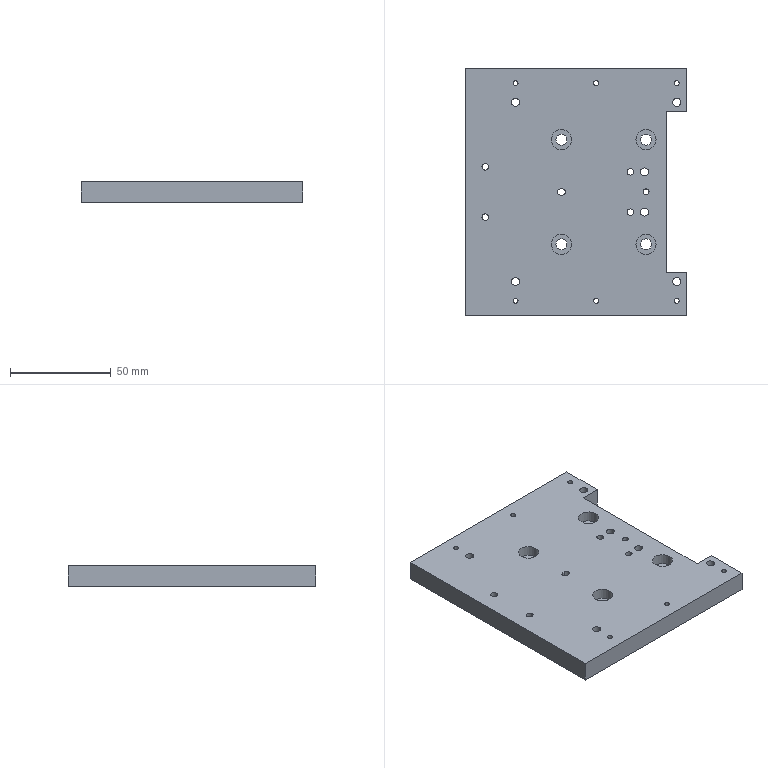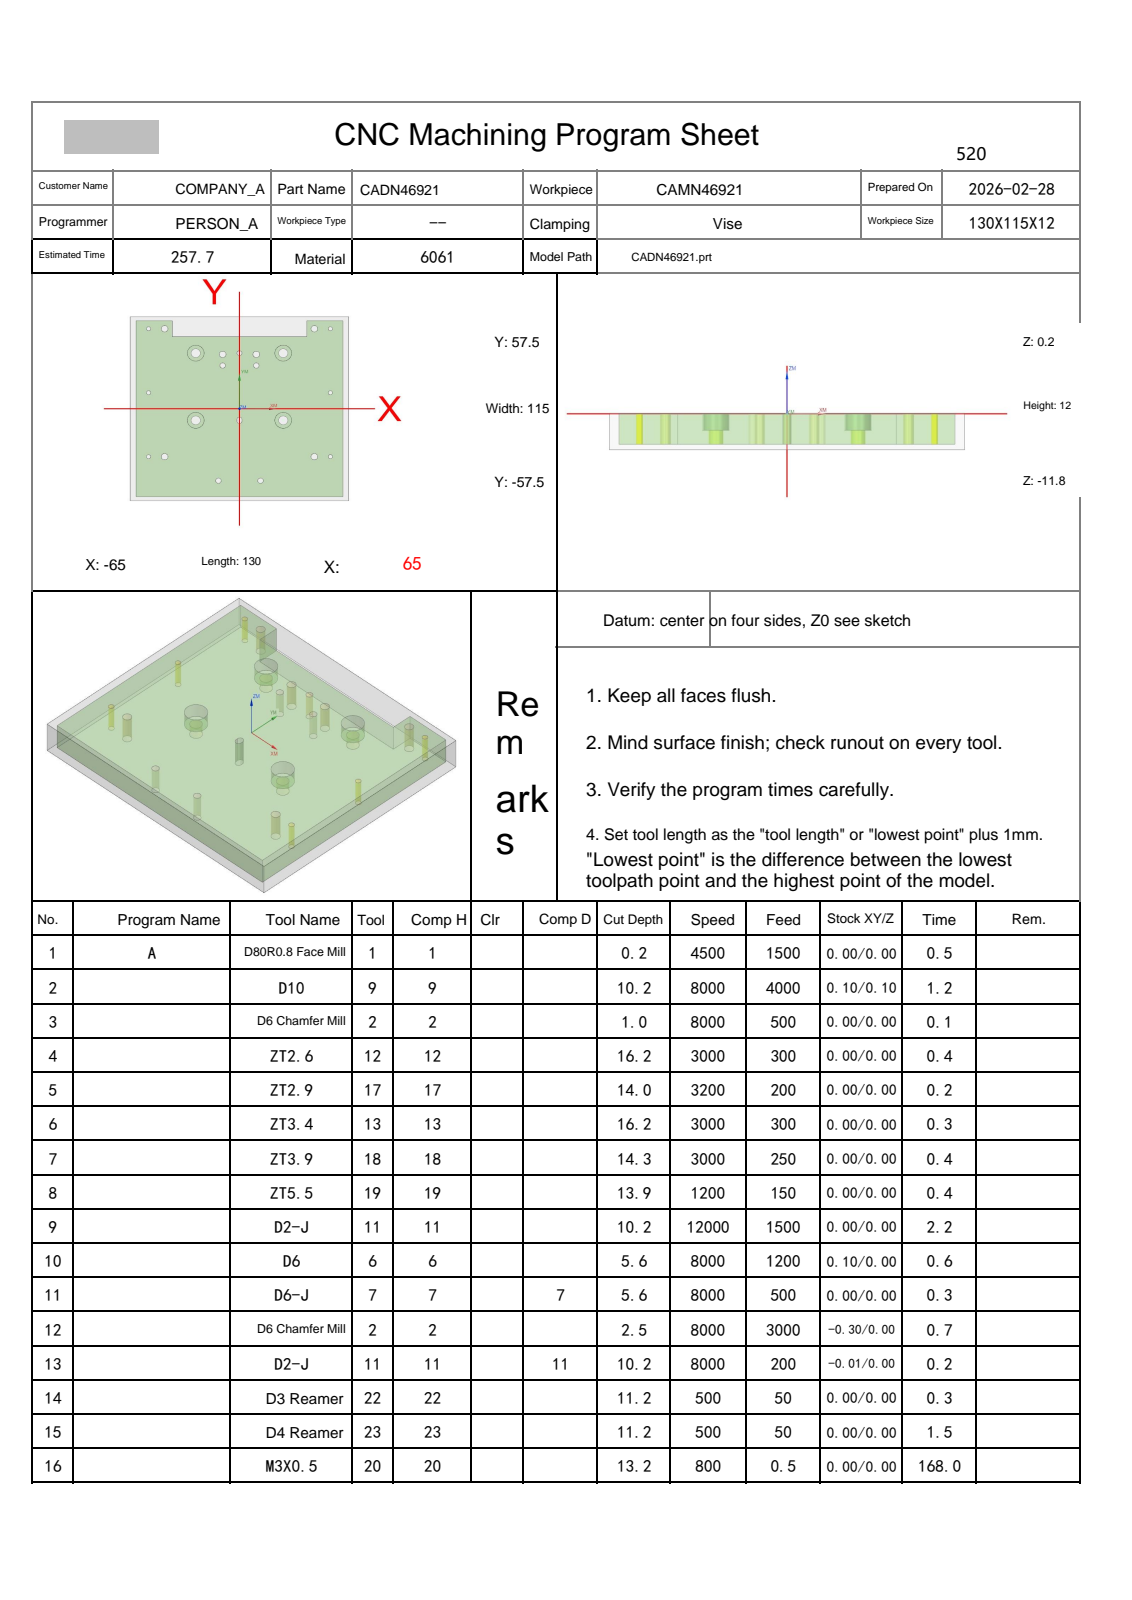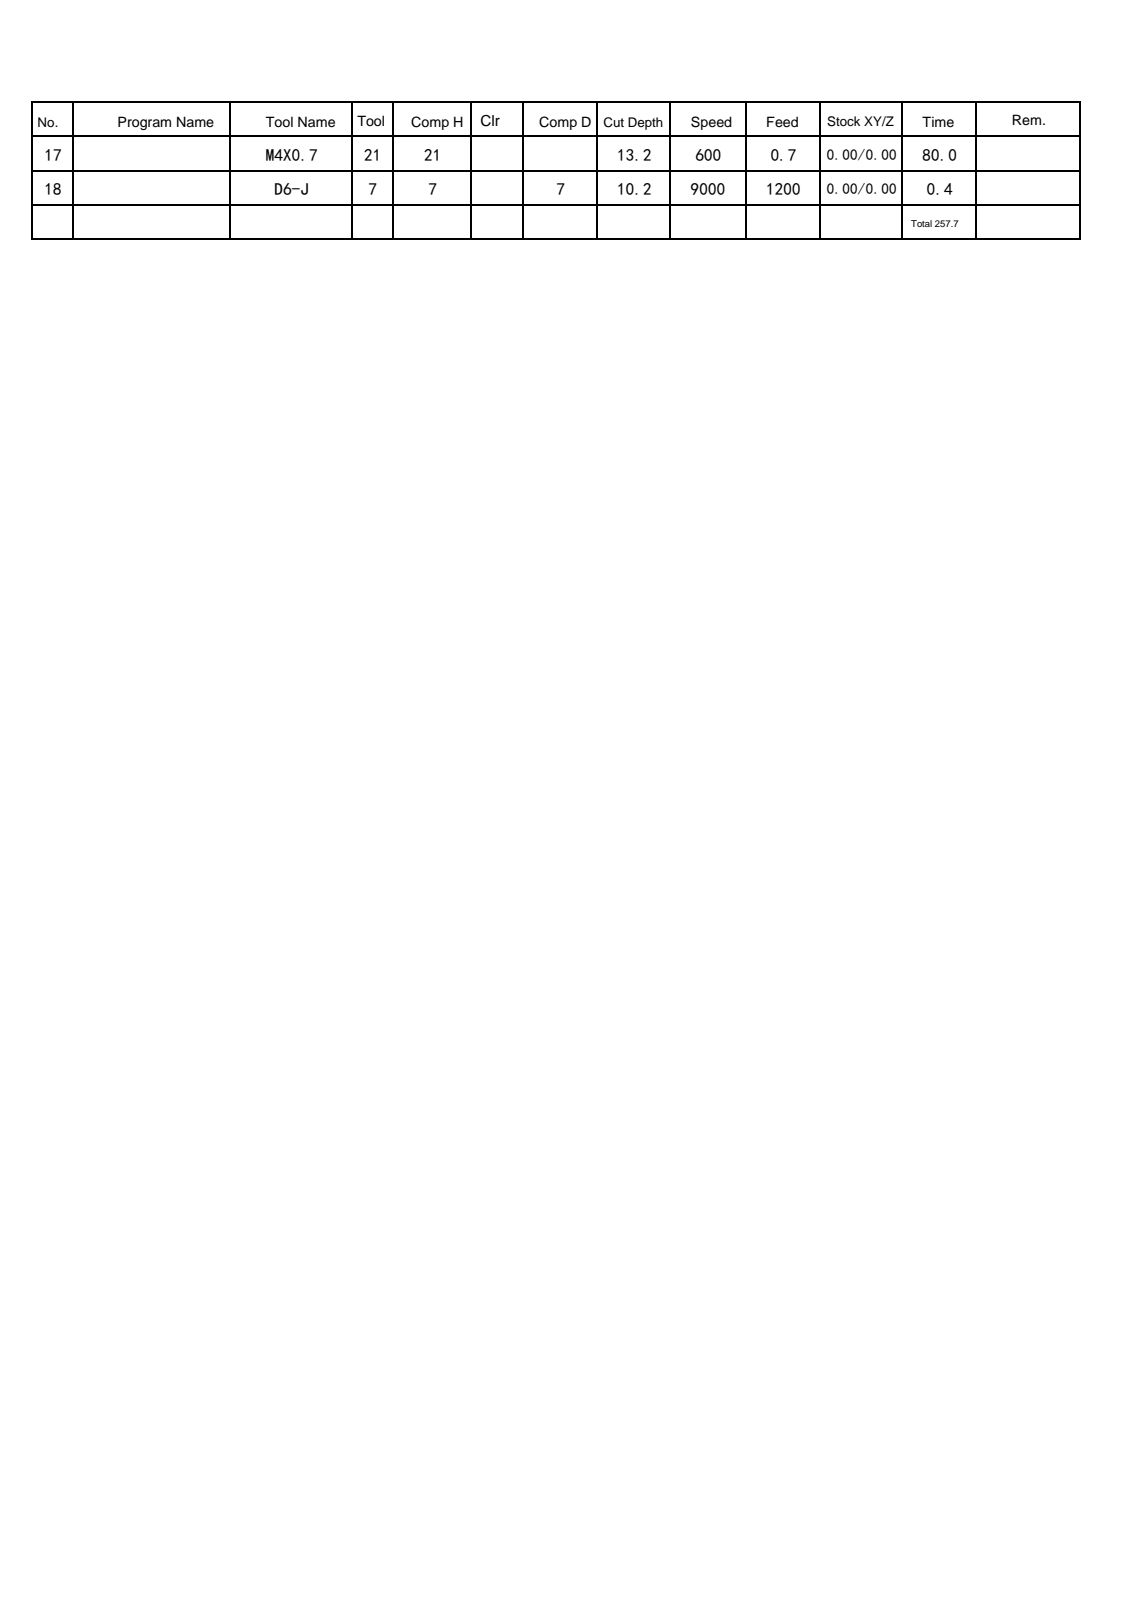NC program | NX | posted by the shop | part box 110 x 123 x 10 mm
Lines 3877 to 4511 of 4511:
N10 T06 M06
(D6  D=6. R=0. H=06 ce=0.10 di=0.00)
G00 G90 G54 X26. Y34.75 M03 S8000
G43 H06 Z50.
M08
Z.5
G03 X26.95 Y35.7 I0.0 J.95 F1200.
X26. Y36.65 I-.95 J0.0
X26. Y36.65 Z0.0 I0.0 J-1.9
X26. Y36.65 Z-.5 I0.0 J-1.9
X26. Y36.65 Z-1. I0.0 J-1.9
X26. Y36.65 Z-1.5 I0.0 J-1.9
X26. Y36.65 Z-2. I0.0 J-1.9
X26. Y36.65 Z-2.5 I0.0 J-1.9
X26. Y36.65 Z-3. I0.0 J-1.9
X26. Y36.65 Z-3.5 I0.0 J-1.9
X26. Y36.65 Z-4. I0.0 J-1.9
X26. Y36.65 Z-4.5 I0.0 J-1.9
X26. Y36.65 Z-5. I0.0 J-1.9
X27.807 Y35.337 Z-5.4 I0.0 J-1.9
X26. Y36.65 I-1.807 J-.587
X24.1 Y34.75 I0.0 J-1.9
X26. Y32.85 I1.9 J0.0
X27.9 Y34.75 I0.0 J1.9
X27.807 Y35.337 I-1.9 J0.0
X26.904 Y35.994 I-.904 J-.294
X25.954 Y35.044 I0.0 J-.95
X26. Y34.75 I.95 J0.0
G00 Z50.
Y-7.25
Z.5
G03 X26.95 Y-6.3 I0.0 J.95
X26. Y-5.35 I-.95 J0.0
X26. Y-5.35 Z0.0 I0.0 J-1.9
X26. Y-5.35 Z-.5 I0.0 J-1.9
X26. Y-5.35 Z-1. I0.0 J-1.9
X26. Y-5.35 Z-1.5 I0.0 J-1.9
X26. Y-5.35 Z-2. I0.0 J-1.9
X26. Y-5.35 Z-2.5 I0.0 J-1.9
X26. Y-5.35 Z-3. I0.0 J-1.9
X26. Y-5.35 Z-3.5 I0.0 J-1.9
X26. Y-5.35 Z-4. I0.0 J-1.9
X26. Y-5.35 Z-4.5 I0.0 J-1.9
X26. Y-5.35 Z-5. I0.0 J-1.9
X27.807 Y-6.663 Z-5.4 I0.0 J-1.9
X26. Y-5.35 I-1.807 J-.587
X24.1 Y-7.25 I0.0 J-1.9
X26. Y-9.15 I1.9 J0.0
X27.9 Y-7.25 I0.0 J1.9
X27.807 Y-6.663 I-1.9 J0.0
X26.904 Y-6.006 I-.904 J-.294
X25.954 Y-6.956 I0.0 J-.95
X26. Y-7.25 I.95 J0.0
G00 Z50.
X-26.
Z.5
G03 X-25.05 Y-6.3 I0.0 J.95
X-26. Y-5.35 I-.95 J0.0
X-26. Y-5.35 Z0.0 I0.0 J-1.9
X-26. Y-5.35 Z-.5 I0.0 J-1.9
X-26. Y-5.35 Z-1. I0.0 J-1.9
X-26. Y-5.35 Z-1.5 I0.0 J-1.9
X-26. Y-5.35 Z-2. I0.0 J-1.9
X-26. Y-5.35 Z-2.5 I0.0 J-1.9
X-26. Y-5.35 Z-3. I0.0 J-1.9
X-26. Y-5.35 Z-3.5 I0.0 J-1.9
X-26. Y-5.35 Z-4. I0.0 J-1.9
X-26. Y-5.35 Z-4.5 I0.0 J-1.9
X-26. Y-5.35 Z-5. I0.0 J-1.9
X-24.193 Y-6.663 Z-5.4 I0.0 J-1.9
X-26. Y-5.35 I-1.807 J-.587
X-27.9 Y-7.25 I0.0 J-1.9
X-26. Y-9.15 I1.9 J0.0
X-24.1 Y-7.25 I0.0 J1.9
X-24.193 Y-6.663 I-1.9 J0.0
X-25.096 Y-6.006 I-.904 J-.294
X-26.046 Y-6.956 I0.0 J-.95
X-26. Y-7.25 I.95 J0.0
G00 Z50.
Y34.75
Z.5
G03 X-25.05 Y35.7 I0.0 J.95
X-26. Y36.65 I-.95 J0.0
X-26. Y36.65 Z0.0 I0.0 J-1.9
X-26. Y36.65 Z-.5 I0.0 J-1.9
X-26. Y36.65 Z-1. I0.0 J-1.9
X-26. Y36.65 Z-1.5 I0.0 J-1.9
X-26. Y36.65 Z-2. I0.0 J-1.9
X-26. Y36.65 Z-2.5 I0.0 J-1.9
X-26. Y36.65 Z-3. I0.0 J-1.9
X-26. Y36.65 Z-3.5 I0.0 J-1.9
X-26. Y36.65 Z-4. I0.0 J-1.9
X-26. Y36.65 Z-4.5 I0.0 J-1.9
X-26. Y36.65 Z-5. I0.0 J-1.9
X-24.193 Y35.337 Z-5.4 I0.0 J-1.9
X-26. Y36.65 I-1.807 J-.587
X-27.9 Y34.75 I0.0 J-1.9
X-26. Y32.85 I1.9 J0.0
X-24.1 Y34.75 I0.0 J1.9
X-24.193 Y35.337 I-1.9 J0.0
X-25.096 Y35.994 I-.904 J-.294
X-26.046 Y35.044 I0.0 J-.95
X-26. Y34.75 I.95 J0.0
G00 Z50.
G91 G28 Z0.0
M05
M09
G91 G28 Z0.0
M01
N11 T07 M06
(D6-J  D=6. R=0. H=07 ce=0.00 di=0.00)
G00 G90 G54 X26. Y34.75 M03 S8000
G43 H07 Z50.
M08
Z0.0
G41 D07
G01 X26.196 Y34.79 F500.
G03 X26.99 Y35.76 I-.196 J.97
X26. Y36.75 I-.99 J0.0
X26. Y36.75 Z-5. I0.0 J-2.
X25.036 Y36.503 Z-5.4 I0.0 J-2.
X24. Y34.75 I.964 J-1.753
X26. Y32.75 I2. J0.0
X28. Y34.75 I0.0 J2.
X26. Y36.75 I-2. J0.0
X25.036 Y36.503 I0.0 J-2.
X24.523 Y35.635 I.477 J-.868
X25.513 Y34.645 I.99 J0.0
X25.809 Y34.69 I0.0 J.99
G01 G40 X26. Y34.75
G00 Z50.
Y-7.25
Z0.0
G41 D07
G01 X26.196 Y-7.21
G03 X26.99 Y-6.24 I-.196 J.97
X26. Y-5.25 I-.99 J0.0
X26. Y-5.25 Z-5. I0.0 J-2.
X25.036 Y-5.497 Z-5.4 I0.0 J-2.
X24. Y-7.25 I.964 J-1.753
X26. Y-9.25 I2. J0.0
X28. Y-7.25 I0.0 J2.
X26. Y-5.25 I-2. J0.0
X25.036 Y-5.497 I0.0 J-2.
X24.523 Y-6.365 I.477 J-.868
X25.513 Y-7.355 I.99 J0.0
X25.809 Y-7.31 I0.0 J.99
G01 G40 X26. Y-7.25
G00 Z50.
X-26.
Z0.0
G41 D07
G01 X-25.804 Y-7.21
G03 X-25.01 Y-6.24 I-.196 J.97
X-26. Y-5.25 I-.99 J0.0
X-26. Y-5.25 Z-5. I0.0 J-2.
X-26.964 Y-5.497 Z-5.4 I0.0 J-2.
X-28. Y-7.25 I.964 J-1.753
X-26. Y-9.25 I2. J0.0
X-24. Y-7.25 I0.0 J2.
X-26. Y-5.25 I-2. J0.0
X-26.964 Y-5.497 I0.0 J-2.
X-27.477 Y-6.365 I.477 J-.868
X-26.487 Y-7.355 I.99 J0.0
X-26.191 Y-7.31 I0.0 J.99
G01 G40 X-26. Y-7.25
G00 Z50.
Y34.75
Z0.0
G41 D07
G01 X-25.804 Y34.79
G03 X-25.01 Y35.76 I-.196 J.97
X-26. Y36.75 I-.99 J0.0
X-26. Y36.75 Z-5. I0.0 J-2.
X-26.964 Y36.503 Z-5.4 I0.0 J-2.
X-28. Y34.75 I.964 J-1.753
X-26. Y32.75 I2. J0.0
X-24. Y34.75 I0.0 J2.
X-26. Y36.75 I-2. J0.0
X-26.964 Y36.503 I0.0 J-2.
X-27.477 Y35.635 I.477 J-.868
X-26.487 Y34.645 I.99 J0.0
X-26.191 Y34.69 I0.0 J.99
G01 G40 X-26. Y34.75
G00 Z50.
G91 G28 Z0.0
M05
M09
G91 G28 Z0.0
M01
N12 T02 M06
(D6 Chamfer Mill  D=6. R=0. H=02 ce=0.00 di=0.00)
G00 G90 G54 X.25 Y-57.128 M03 S8000
G43 H02 Z50.
M08
Z2.099
G01 Z-1.5 F3000.
G03 X.33 Y-56.828 I-.52 J.3
X.03 Y-56.308 I-.6 J0.0
G01 X0.0 Y-56.3
X-61.5
G02 X-62.8 Y-55. I0.0 J1.3
G01 Y55.
G02 X-61.5 Y56.3 I1.3 J0.0
G01 X-40.
G02 X-38.7 Y55. I0.0 J-1.3
G01 Y46.3
X38.7
Y55.
G02 X40. Y56.3 I1.3 J0.0
G01 X61.5
G02 X62.8 Y55. I0.0 J-1.3
G01 Y-55.
G02 X61.5 Y-56.3 I-1.3 J0.0
G01 X0.0
X-.03 Y-56.308
G03 X-.33 Y-56.828 I.3 J-.52
X-.25 Y-57.128 I.6 J0.0
G01 Z2.099
G00 Z50.
X-.214 Y-7.375
Z2.941
G01 Z-1.5
X-.064 Y-7.415
G03 X.196 Y-7.265 I0.0 J.3
G01 X.2 Y-7.25
Y-6.75
X.173 Y-6.65
X.1 Y-6.577
X0.0 Y-6.55
X-.1 Y-6.577
X-.173 Y-6.65
X-.2 Y-6.75
Y-7.75
X-.173 Y-7.85
X-.1 Y-7.923
X0.0 Y-7.95
X.1 Y-7.923
X.173 Y-7.85
X.2 Y-7.75
Y-7.25
X.196 Y-7.235
G03 X-.064 Y-7.085 I-.26 J-.15
G01 X-.214 Y-7.125
Z2.941
G00 Z50.
G00 G90 X54. Y50. M03 S8000
Z50.
G98 G81 X54. Y50. Z-1.75 R3. F500.
Y10.
Y-30.
X-54.
Y10.
Y50.
G80
G00 Z50.
G00 G90 X0.0 Y34.75 M03 S8000
Z50.
G98 G81 X0.0 Y34.75 Z-1.8 R3. F500.
G80
G00 Z50.
G00 G90 X12.5 Y-45. M03 S8000
Z50.
G98 G81 X12.5 Y-45. Z-2.2 R3. F500.
X-12.5
X-10. Y27.
X10.
G80
G00 Z50.
G00 G90 X44.5 Y-30. M03 S8000
Z50.
G98 G81 X44.5 Y-30. Z-2.3 R3. F500.
Y50.
X10. Y34.
X-10.
X-44.5 Y50.
Y-30.
G80
G00 Z50.
G00 G90 X-22.614 Y32.096 M03 S8000
Z50.
Z2.5
G01 X-22.606 Y32.105 Z2.495 F800.
X-22.356 Y32.461 Z2.337
X-22.196 Y32.739 Z2.22
X-22.012 Y33.133 Z2.062
X-21.87 Y33.543 Z1.904
X-21.769 Y33.966 Z1.746
X-21.712 Y34.396 Z1.588
X-21.698 Y34.83 Z1.43
X-21.728 Y35.264 Z1.272
X-21.801 Y35.692 Z1.114
X-21.918 Y36.11 Z.956
X-22.076 Y36.515 Z.797
X-22.273 Y36.902 Z.639
X-22.509 Y37.266 Z.481
X-22.781 Y37.605 Z.323
X-23.085 Y37.915 Z.165
X-23.419 Y38.193 Z.007
X-23.779 Y38.436 Z-.151
X-24.162 Y38.641 Z-.309
X-24.564 Y38.806 Z-.467
X-24.98 Y38.93 Z-.625
X-25.407 Y39.012 Z-.783
X-25.839 Y39.05 Z-.942
X-26. Z-1.
G03 X-30.3 Y34.75 I0.0 J-4.3
X-26. Y30.45 I4.3 J0.0
X-21.7 Y34.75 I0.0 J4.3
X-26. Y39.05 I-4.3 J0.0
X-26.499 Y39.021 I0.0 J-4.3
G01 Z1.5
G00 Z50.
X-22.614 Y-9.904
Z2.5
G01 X-22.606 Y-9.895 Z2.495
X-22.356 Y-9.539 Z2.337
X-22.196 Y-9.261 Z2.22
X-22.012 Y-8.867 Z2.062
X-21.87 Y-8.457 Z1.904
X-21.769 Y-8.034 Z1.746
X-21.712 Y-7.604 Z1.588
X-21.698 Y-7.17 Z1.43
X-21.728 Y-6.736 Z1.272
X-21.801 Y-6.308 Z1.114
X-21.918 Y-5.89 Z.956
X-22.076 Y-5.485 Z.797
X-22.273 Y-5.099 Z.639
X-22.509 Y-4.734 Z.481
X-22.781 Y-4.395 Z.323
X-23.085 Y-4.085 Z.165
X-23.419 Y-3.807 Z.007
X-23.779 Y-3.564 Z-.151
X-24.162 Y-3.359 Z-.309
X-24.564 Y-3.194 Z-.467
X-24.98 Y-3.07 Z-.625
X-25.407 Y-2.988 Z-.783
X-25.839 Y-2.95 Z-.942
X-26. Z-1.
G03 X-30.3 Y-7.25 I0.0 J-4.3
X-26. Y-11.55 I4.3 J0.0
X-21.7 Y-7.25 I0.0 J4.3
X-26. Y-2.95 I-4.3 J0.0
X-26.499 Y-2.979 I0.0 J-4.3
G01 Z1.5
G00 Z50.
X29.386 Y-9.904
Z2.5
G01 X29.394 Y-9.895 Z2.495
X29.644 Y-9.539 Z2.337
X29.804 Y-9.261 Z2.22
X29.988 Y-8.867 Z2.062
X30.13 Y-8.457 Z1.904
X30.231 Y-8.034 Z1.746
X30.288 Y-7.604 Z1.588
X30.302 Y-7.17 Z1.43
X30.272 Y-6.736 Z1.272
X30.199 Y-6.308 Z1.114
X30.082 Y-5.89 Z.956
X29.924 Y-5.485 Z.797
X29.727 Y-5.099 Z.639
X29.491 Y-4.734 Z.481
X29.219 Y-4.395 Z.323
X28.915 Y-4.085 Z.165
X28.581 Y-3.807 Z.007
X28.221 Y-3.564 Z-.151
X27.838 Y-3.359 Z-.309
X27.436 Y-3.194 Z-.467
X27.02 Y-3.07 Z-.625
X26.593 Y-2.988 Z-.783
X26.161 Y-2.95 Z-.942
X26. Z-1.
G03 X21.7 Y-7.25 I0.0 J-4.3
X26. Y-11.55 I4.3 J0.0
X30.3 Y-7.25 I0.0 J4.3
X26. Y-2.95 I-4.3 J0.0
X25.501 Y-2.979 I0.0 J-4.3
G01 Z1.5
G00 Z50.
X29.386 Y32.096
Z2.5
G01 X29.394 Y32.105 Z2.495
X29.644 Y32.461 Z2.337
X29.804 Y32.739 Z2.22
X29.988 Y33.133 Z2.062
X30.13 Y33.543 Z1.904
X30.231 Y33.966 Z1.746
X30.288 Y34.396 Z1.588
X30.302 Y34.83 Z1.43
X30.272 Y35.264 Z1.272
X30.199 Y35.692 Z1.114
X30.082 Y36.11 Z.956
X29.924 Y36.515 Z.797
X29.727 Y36.902 Z.639
X29.491 Y37.266 Z.481
X29.219 Y37.605 Z.323
X28.915 Y37.915 Z.165
X28.581 Y38.193 Z.007
X28.221 Y38.436 Z-.151
X27.838 Y38.641 Z-.309
X27.436 Y38.806 Z-.467
X27.02 Y38.93 Z-.625
X26.593 Y39.012 Z-.783
X26.161 Y39.05 Z-.942
X26. Z-1.
G03 X21.7 Y34.75 I0.0 J-4.3
X26. Y30.45 I4.3 J0.0
X30.3 Y34.75 I0.0 J4.3
X26. Y39.05 I-4.3 J0.0
X25.501 Y39.021 I0.0 J-4.3
G01 Z1.5
G00 Z50.
G91 G28 Z0.0
M05
M09
G91 G28 Z0.0
M01
N13 T11 M06
(D2-J  D=2. R=0. H=11 ce=-0.01 di=0.00)
G00 G90 G54 X.26 Y-7.406 M03 S8000
G43 H11 Z50.
M08
Z-1.5
G01 Z-2. F200.
G41 D11
X.31
G03 X.51 Y-7.206 I0.0 J.2
G01 Y-6.75
G03 X0.0 Y-6.24 I-.51 J0.0
X-.51 Y-6.75 I0.0 J-.51
G01 Y-7.75
G03 X0.0 Y-8.26 I.51 J0.0
X.51 Y-7.75 I0.0 J.51
G01 Y-7.206
Y-6.75
X.508 Y-6.706
G03 X.309 Y-6.523 I-.199 J-.017
G01 X.292 Y-6.524
X.219 Y-6.53
G40 X.169 Y-6.535
Z-1.5
G00 Z.5
X.26 Y-7.406
Z-3.5
G01 Z-4.
G41 D11
X.31
G03 X.51 Y-7.206 I0.0 J.2
G01 Y-6.75
G03 X0.0 Y-6.24 I-.51 J0.0
X-.51 Y-6.75 I0.0 J-.51
G01 Y-7.75
G03 X0.0 Y-8.26 I.51 J0.0
X.51 Y-7.75 I0.0 J.51
G01 Y-7.206
Y-6.75
X.508 Y-6.706
G03 X.309 Y-6.523 I-.199 J-.017
G01 X.292 Y-6.524
X.219 Y-6.53
G40 X.169 Y-6.535
Z-3.5
G00 Z-1.5
X.26 Y-7.406
Z-5.5
G01 Z-6.
G41 D11
X.31
G03 X.51 Y-7.206 I0.0 J.2
G01 Y-6.75
G03 X0.0 Y-6.24 I-.51 J0.0
X-.51 Y-6.75 I0.0 J-.51
G01 Y-7.75
G03 X0.0 Y-8.26 I.51 J0.0
X.51 Y-7.75 I0.0 J.51
G01 Y-7.206
Y-6.75
X.508 Y-6.706
G03 X.309 Y-6.523 I-.199 J-.017
G01 X.292 Y-6.524
X.219 Y-6.53
G40 X.169 Y-6.535
Z-5.5
G00 Z-3.5
X.26 Y-7.406
Z-7.5
G01 Z-8.
G41 D11
X.31
G03 X.51 Y-7.206 I0.0 J.2
G01 Y-6.75
G03 X0.0 Y-6.24 I-.51 J0.0
X-.51 Y-6.75 I0.0 J-.51
G01 Y-7.75
G03 X0.0 Y-8.26 I.51 J0.0
X.51 Y-7.75 I0.0 J.51
G01 Y-7.206
Y-6.75
X.508 Y-6.706
G03 X.309 Y-6.523 I-.199 J-.017
G01 X.292 Y-6.524
X.219 Y-6.53
G40 X.169 Y-6.535
Z-7.5
G00 Z-5.5
X.26 Y-7.406
Z-9.5
G01 Z-10.
G41 D11
X.31
G03 X.51 Y-7.206 I0.0 J.2
G01 Y-6.75
G03 X0.0 Y-6.24 I-.51 J0.0
X-.51 Y-6.75 I0.0 J-.51
G01 Y-7.75
G03 X0.0 Y-8.26 I.51 J0.0
X.51 Y-7.75 I0.0 J.51
G01 Y-7.206
Y-6.75
X.508 Y-6.706
G03 X.309 Y-6.523 I-.199 J-.017
G01 X.292 Y-6.524
X.219 Y-6.53
G40 X.169 Y-6.535
Z-9.5
G00 Z50.
G91 G28 Z0.0
M05
M09
G91 G28 Z0.0
M01
N14 T22 M06
(D3 Reamer D=3. DR_a=180 H=22)
G00 G90 G54 X0.0 Y34.75 M03 S500
G43 H22 Z50.
M08
G98 G81 X0.0 Y34.75 Z-11. R1. F50.
G80
G00 Z50.
G91 G28 Z0.0
M05
M09
G91 G28 Z0.0
M01
N15 T23 M06
(D4 Reamer D=4. DR_a=180 H=23)
G00 G90 G54 X44.5 Y-30. M03 S500
G43 H23 Z50.
M08
G98 G81 X44.5 Y-30. Z-11. R1. F50.
Y50.
X10. Y34.
X-10.
X-44.5 Y50.
Y-30.
G80
G00 Z50.
G91 G28 Z0.0
M05
M09
G91 G28 Z0.0
M01
N16 T20 M06
(M3X0.5 D=2.5 DR_a=180 H=20)
G00 G90 G54 X54. Y50. M03 S800
G43 H20 Z50.
M08
G95
G98 G84 X54. Y50. Z-13. R1. F.5 Q5.
Y10.
Y-30.
X-54.
Y10.
Y50.
G80
G94
G00 Z50.
G91 G28 Z0.0
M05
M09
G91 G28 Z0.0
M01
N17 T21 M06
(M4X0.7 D=3.3 DR_a=180 H=21)
G00 G90 G54 X12.5 Y-45. M03 S600
G43 H21 Z50.
M08
G95
G98 G84 X12.5 Y-45. Z-13. R1. F.7 Q4.
X-12.5
X-10. Y27.
X10.
G80
G94
G00 Z50.
G91 G28 Z0.0
M05
M09
G91 G28 Z0.0
M01
N18 T07 M06
(D6-J  D=6. R=0. H=07 ce=0.00 di=0.00)
G00 G90 G54 X62.517 Y-59.073 M03 S9000
G43 H07 Z50.
M08
Z-9.5
G01 Z-10. F1200.
G41 D07
X62.492 Y-58.875
G03 X61.5 Y-58. I-.992 J-.125
G01 X-61.5
G02 X-64.5 Y-55. I0.0 J3.
G01 Y55.
G02 X-61.5 Y58. I3. J0.0
G01 X-40.
G02 X-37. Y55. I0.0 J-3.
G01 Y48.
X37.
Y55.
G02 X40. Y58. I3. J0.0
G01 X61.5
G02 X64.5 Y55. I0.0 J-3.
G01 Y-55.
G02 X61.5 Y-58. I-3. J0.0
G01 X61.
G03 X60. Y-59. I0.0 J-1.
G01 G40 Y-59.2
Z-9.5
G00 Z50.
M05
M09
G91 G28 Z0.0
G91 G28 Y0.0
M30
%